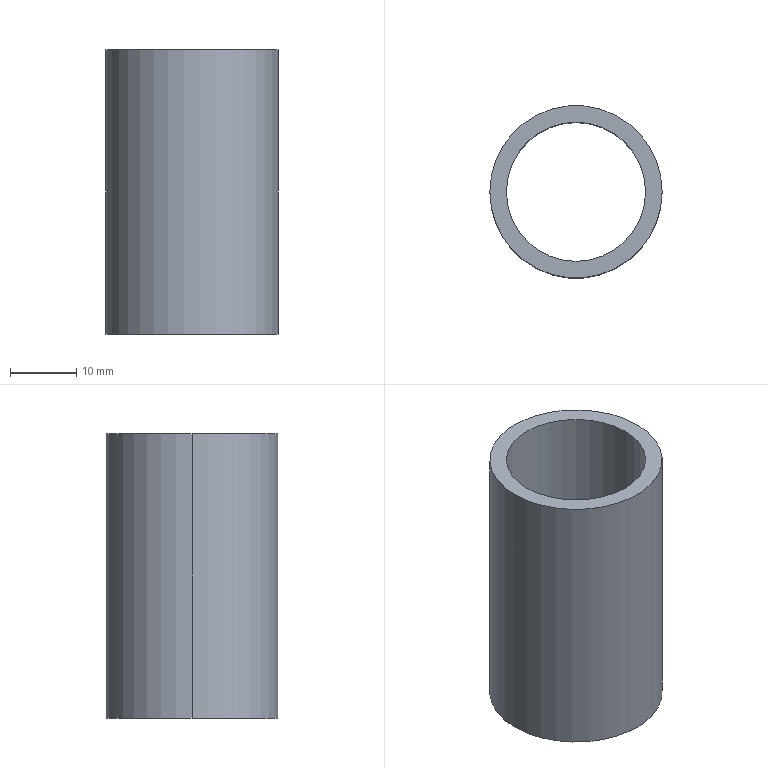Part | SolidWorks | features ICE 1, LibraryFeature 1 | 1 solid | 6 faces | box 26 x 26 x 43 mm | volume 7936 mm3 | cylinder 4 | plane 2 | commonest cylinder face diameters 21 x2 26 x2
STEP:
#1=CARTESIAN_POINT('',(-10.5,0.,21.5));
#2=VERTEX_POINT('',#1);
#3=CARTESIAN_POINT('',(10.5,0.,21.5));
#4=VERTEX_POINT('',#3);
#5=CARTESIAN_POINT('',(0.,0.,21.5));
#6=DIRECTION('',(0.,0.,1.));
#7=DIRECTION('',(1.,0.,0.));
#8=AXIS2_PLACEMENT_3D('',#5,#6,#7);
#9=CIRCLE('',#8,10.5);
#10=EDGE_CURVE('',#2,#4,#9,.T.);
#11=ORIENTED_EDGE('',*,*,#10,.T.);
#12=CARTESIAN_POINT('',(10.5,0.,-21.5));
#13=VERTEX_POINT('',#12);
#14=CARTESIAN_POINT('',(10.5,0.,21.5));
#15=DIRECTION('',(0.,0.,-1.));
#16=VECTOR('',#15,1000.);
#17=LINE('',#14,#16);
#18=EDGE_CURVE('',#4,#13,#17,.T.);
#19=ORIENTED_EDGE('',*,*,#18,.T.);
#20=CARTESIAN_POINT('',(-10.5,0.,-21.5));
#21=VERTEX_POINT('',#20);
#22=CARTESIAN_POINT('',(0.,0.,-21.5));
#23=DIRECTION('',(0.,0.,1.));
#24=DIRECTION('',(1.,0.,0.));
#25=AXIS2_PLACEMENT_3D('',#22,#23,#24);
#26=CIRCLE('',#25,10.5);
#27=EDGE_CURVE('',#21,#13,#26,.T.);
#28=ORIENTED_EDGE('',*,*,#27,.F.);
#29=CARTESIAN_POINT('',(-10.5,0.,21.5));
#30=DIRECTION('',(0.,0.,-1.));
#31=VECTOR('',#30,1000.);
#32=LINE('',#29,#31);
#33=EDGE_CURVE('',#2,#21,#32,.T.);
#34=ORIENTED_EDGE('',*,*,#33,.F.);
#35=EDGE_LOOP('',(#11,#19,#28,#34));
#36=FACE_OUTER_BOUND('',#35,.T.);
#37=CARTESIAN_POINT('',(0.,0.,21.5));
#38=DIRECTION('',(0.,0.,-1.));
#39=DIRECTION('',(-1.,0.,0.));
#40=AXIS2_PLACEMENT_3D('',#37,#38,#39);
#41=CYLINDRICAL_SURFACE('',#40,10.5);
#42=ADVANCED_FACE('',(#36),#41,.F.);
#43=CARTESIAN_POINT('',(13.,0.,21.5));
#44=VERTEX_POINT('',#43);
#45=CARTESIAN_POINT('',(-13.,0.,21.5));
#46=VERTEX_POINT('',#45);
#47=CARTESIAN_POINT('',(0.,0.,21.5));
#48=DIRECTION('',(0.,0.,1.));
#49=DIRECTION('',(1.,0.,0.));
#50=AXIS2_PLACEMENT_3D('',#47,#48,#49);
#51=CIRCLE('',#50,13.);
#52=EDGE_CURVE('',#44,#46,#51,.T.);
#53=ORIENTED_EDGE('',*,*,#52,.F.);
#54=CARTESIAN_POINT('',(13.,0.,-21.5));
#55=VERTEX_POINT('',#54);
#56=CARTESIAN_POINT('',(13.,0.,21.5));
#57=DIRECTION('',(0.,0.,-1.));
#58=VECTOR('',#57,1000.);
#59=LINE('',#56,#58);
#60=EDGE_CURVE('',#44,#55,#59,.T.);
#61=ORIENTED_EDGE('',*,*,#60,.T.);
#62=CARTESIAN_POINT('',(-13.,0.,-21.5));
#63=VERTEX_POINT('',#62);
#64=CARTESIAN_POINT('',(0.,0.,-21.5));
#65=DIRECTION('',(0.,0.,1.));
#66=DIRECTION('',(1.,0.,0.));
#67=AXIS2_PLACEMENT_3D('',#64,#65,#66);
#68=CIRCLE('',#67,13.);
#69=EDGE_CURVE('',#55,#63,#68,.T.);
#70=ORIENTED_EDGE('',*,*,#69,.T.);
#71=CARTESIAN_POINT('',(-13.,0.,21.5));
#72=DIRECTION('',(0.,0.,-1.));
#73=VECTOR('',#72,1000.);
#74=LINE('',#71,#73);
#75=EDGE_CURVE('',#46,#63,#74,.T.);
#76=ORIENTED_EDGE('',*,*,#75,.F.);
#77=EDGE_LOOP('',(#53,#61,#70,#76));
#78=FACE_OUTER_BOUND('',#77,.T.);
#79=CARTESIAN_POINT('',(0.,0.,21.5));
#80=DIRECTION('',(0.,0.,-1.));
#81=DIRECTION('',(-1.,0.,0.));
#82=AXIS2_PLACEMENT_3D('',#79,#80,#81);
#83=CYLINDRICAL_SURFACE('',#82,13.);
#84=ADVANCED_FACE('',(#78),#83,.T.);
#85=CARTESIAN_POINT('',(0.,0.,21.5));
#86=DIRECTION('',(0.,0.,1.));
#87=DIRECTION('',(1.,0.,0.));
#88=AXIS2_PLACEMENT_3D('',#85,#86,#87);
#89=CIRCLE('',#88,13.);
#90=EDGE_CURVE('',#46,#44,#89,.T.);
#91=ORIENTED_EDGE('',*,*,#90,.T.);
#92=ORIENTED_EDGE('',*,*,#52,.T.);
#93=EDGE_LOOP('',(#91,#92));
#94=FACE_OUTER_BOUND('',#93,.T.);
#95=ORIENTED_EDGE('',*,*,#10,.F.);
#96=CARTESIAN_POINT('',(0.,0.,21.5));
#97=DIRECTION('',(0.,0.,1.));
#98=DIRECTION('',(1.,0.,0.));
#99=AXIS2_PLACEMENT_3D('',#96,#97,#98);
#100=CIRCLE('',#99,10.5);
#101=EDGE_CURVE('',#4,#2,#100,.T.);
#102=ORIENTED_EDGE('',*,*,#101,.F.);
#103=EDGE_LOOP('',(#95,#102));
#104=FACE_BOUND('',#103,.T.);
#105=CARTESIAN_POINT('',(0.,0.,21.5));
#106=DIRECTION('',(0.,0.,1.));
#107=DIRECTION('',(1.,0.,0.));
#108=AXIS2_PLACEMENT_3D('',#105,#106,#107);
#109=PLANE('',#108);
#110=ADVANCED_FACE('',(#94,#104),#109,.T.);
#111=CARTESIAN_POINT('',(0.,0.,-21.5));
#112=DIRECTION('',(0.,0.,1.));
#113=DIRECTION('',(1.,0.,0.));
#114=AXIS2_PLACEMENT_3D('',#111,#112,#113);
#115=CIRCLE('',#114,13.);
#116=EDGE_CURVE('',#63,#55,#115,.T.);
#117=ORIENTED_EDGE('',*,*,#116,.F.);
#118=ORIENTED_EDGE('',*,*,#69,.F.);
#119=EDGE_LOOP('',(#117,#118));
#120=FACE_OUTER_BOUND('',#119,.T.);
#121=ORIENTED_EDGE('',*,*,#27,.T.);
#122=CARTESIAN_POINT('',(0.,0.,-21.5));
#123=DIRECTION('',(0.,0.,1.));
#124=DIRECTION('',(1.,0.,0.));
#125=AXIS2_PLACEMENT_3D('',#122,#123,#124);
#126=CIRCLE('',#125,10.5);
#127=EDGE_CURVE('',#13,#21,#126,.T.);
#128=ORIENTED_EDGE('',*,*,#127,.T.);
#129=EDGE_LOOP('',(#121,#128));
#130=FACE_BOUND('',#129,.T.);
#131=CARTESIAN_POINT('',(0.,0.,-21.5));
#132=DIRECTION('',(0.,0.,1.));
#133=DIRECTION('',(1.,0.,0.));
#134=AXIS2_PLACEMENT_3D('',#131,#132,#133);
#135=PLANE('',#134);
#136=ADVANCED_FACE('',(#120,#130),#135,.F.);
#137=ORIENTED_EDGE('',*,*,#60,.F.);
#138=ORIENTED_EDGE('',*,*,#90,.F.);
#139=ORIENTED_EDGE('',*,*,#75,.T.);
#140=ORIENTED_EDGE('',*,*,#116,.T.);
#141=EDGE_LOOP('',(#137,#138,#139,#140));
#142=FACE_OUTER_BOUND('',#141,.T.);
#143=CARTESIAN_POINT('',(0.,0.,21.5));
#144=DIRECTION('',(0.,0.,-1.));
#145=DIRECTION('',(-1.,0.,0.));
#146=AXIS2_PLACEMENT_3D('',#143,#144,#145);
#147=CYLINDRICAL_SURFACE('',#146,13.);
#148=ADVANCED_FACE('',(#142),#147,.T.);
#149=ORIENTED_EDGE('',*,*,#18,.F.);
#150=ORIENTED_EDGE('',*,*,#101,.T.);
#151=ORIENTED_EDGE('',*,*,#33,.T.);
#152=ORIENTED_EDGE('',*,*,#127,.F.);
#153=EDGE_LOOP('',(#149,#150,#151,#152));
#154=FACE_OUTER_BOUND('',#153,.T.);
#155=CARTESIAN_POINT('',(0.,0.,21.5));
#156=DIRECTION('',(0.,0.,-1.));
#157=DIRECTION('',(-1.,0.,0.));
#158=AXIS2_PLACEMENT_3D('',#155,#156,#157);
#159=CYLINDRICAL_SURFACE('',#158,10.5);
#160=ADVANCED_FACE('',(#154),#159,.F.);
#161=CLOSED_SHELL('',(#42,#84,#110,#136,#148,#160));
#162=MANIFOLD_SOLID_BREP('',#161);
#163=CARTESIAN_POINT('',(0.,0.,0.));
#164=DIRECTION('',(0.,0.,1.));
#165=DIRECTION('',(1.,0.,0.));
#166=AXIS2_PLACEMENT_3D('',#163,#164,#165);
#167=(LENGTH_UNIT()NAMED_UNIT(*)SI_UNIT(.MILLI.,.METRE.));
#168=UNCERTAINTY_MEASURE_WITH_UNIT(LENGTH_MEASURE(0.00001),#167,'','');
#169=(NAMED_UNIT(*)PLANE_ANGLE_UNIT()SI_UNIT($,.RADIAN.));
#170=(NAMED_UNIT(*)SI_UNIT($,.STERADIAN.)SOLID_ANGLE_UNIT());
#171=(GEOMETRIC_REPRESENTATION_CONTEXT(3)GLOBAL_UNCERTAINTY_ASSIGNED_CONTEXT((#168))GLOBAL_UNIT_ASSIGNED_CONTEXT((#167,#169,#170))REPRESENTATION_CONTEXT('',''));
#172=ADVANCED_BREP_SHAPE_REPRESENTATION('',(#162,#166),#171);